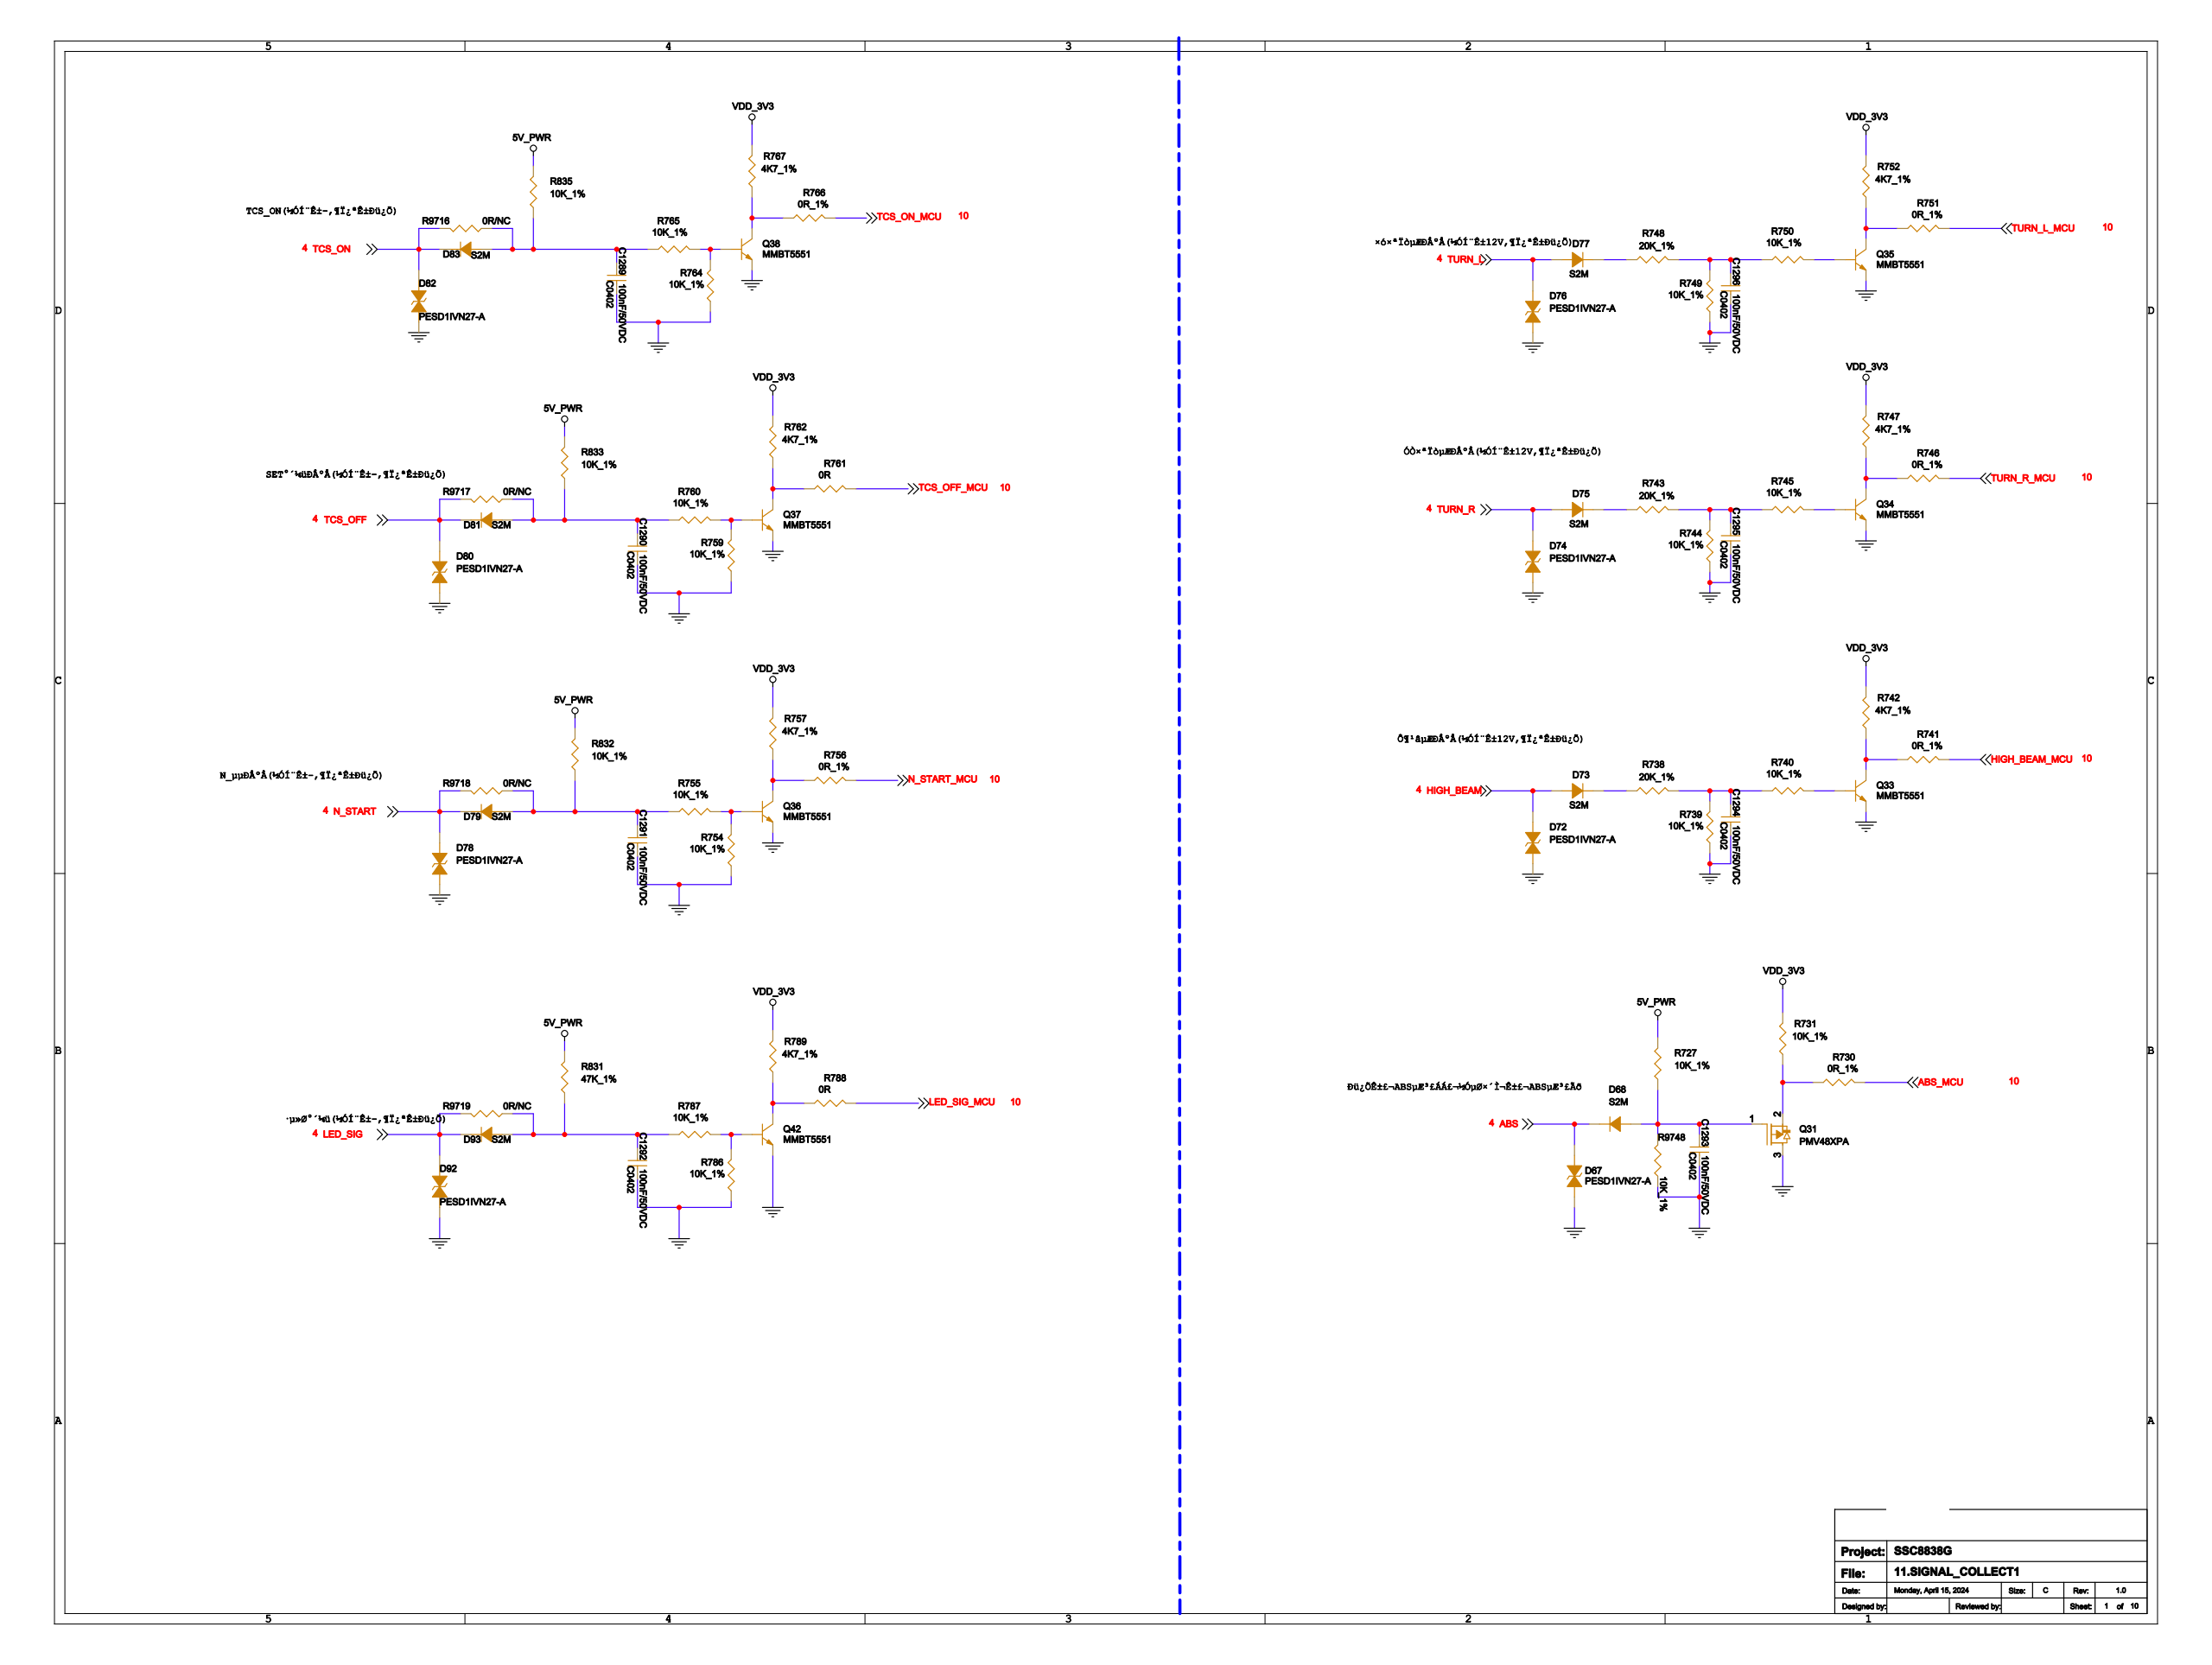Circuit board | Cadence Allegro | 958 parts | 601 nets | one sheet of the schematic
Parts on this sheet (reference | value | footprint):
C1289 | 100nF/50VDC | C0402
C1290 | 100nF/50VDC | C0402
C1291 | 100nF/50VDC | C0402
C1292 | 100nF/50VDC | C0402
C1293 | 100nF/50VDC | C0402
C1294 | 100nF/50VDC | C0402
C1295 | 100nF/50VDC | C0402
C1296 | 100nF/50VDC | C0402
D67 | PESD1IVN27-A | SOD_323
D68 | S2M | DO-214AA
D72 | PESD1IVN27-A | SOD_323
D73 | S2M | DO-214AA
D74 | PESD1IVN27-A | SOD_323
D75 | S2M | DO-214AA
D76 | PESD1IVN27-A | SOD_323
D77 | S2M | DO-214AA
D78 | PESD1IVN27-A | SOD_323
D79 | S2M | DO-214AA
D80 | PESD1IVN27-A | SOD_323
D81 | S2M | DO-214AA
D82 | PESD1IVN27-A | SOD_323
D83 | S2M | DO-214AA
D92 | PESD1IVN27-A | SOD_323
D93 | S2M | DO-214AA
Q31 | PMV48XPA | SOT23-123
Q33 | MMBT5551 | SOT23-123
Q34 | MMBT5551 | SOT23-123
Q35 | MMBT5551 | SOT23-123
Q36 | MMBT5551 | SOT23-123
Q37 | MMBT5551 | SOT23-123
Q38 | MMBT5551 | SOT23-123
Q42 | MMBT5551 | SOT23-123
R727 | 10K_1% | R0402
R730 | 0R_1% | R0402
R731 | 10K_1% | R0402
R738 | 20K_1% | R0402
R739 | 10K_1% | R0402
R740 | 10K_1% | R0402
R741 | 0R_1% | R0402
R742 | 4K7_1% | R0402
R743 | 20K_1% | R0402
R744 | 10K_1% | R0402
R745 | 10K_1% | R0402
R746 | 0R_1% | R0402
R747 | 4K7_1% | R0402
R748 | 20K_1% | R0402
R749 | 10K_1% | R0402
R750 | 10K_1% | R0402
R751 | 0R_1% | R0402
R752 | 4K7_1% | R0402
R754 | 10K_1% | R0402
R755 | 10K_1% | R0402
R756 | 0R_1% | R0402
R757 | 4K7_1% | R0402
R759 | 10K_1% | R0402
R760 | 10K_1% | R0402
R761 | 0R | R0402
R762 | 4K7_1% | R0402
R764 | 10K_1% | R0402
R765 | 10K_1% | R0402
R766 | 0R_1% | R0402
R767 | 4K7_1% | R0402
R786 | 10K_1% | R0402
R787 | 10K_1% | R0402
R788 | 0R | R0402
R789 | 4K7_1% | R0402
R831 | 47K_1% | R0402
R832 | 10K_1% | R0402
R833 | 10K_1% | R0402
R835 | 10K_1% | R0402
R9716 | 0R/NC | R0402
R9717 | 0R/NC | R0402
R9718 | 0R/NC | R0402
R9719 | 0R/NC | R0402
R9748 | 10K_1% | R0402
Nets of these parts (net: part-pin ...):
GND: C1289-2 C1290-2 C1291-2 C1292-2 C1293-2 C1294-2 C1295-2 C1296-2 D67-1 D72-1 D74-1 D76-1 D78-1 D80-1 D82-1 D92-1 Q31-3 Q33-2 Q34-2 Q35-2 Q36-2 Q37-2 Q38-2 Q42-2 R739-1 R744-1 R749-1 R754-1 R759-1 R764-1 R786-1 R9748-1
5V_PWR: R727-2 R831-2 R832-2 R833-2 R835-2
3V3_NORMAL: R731-2 R742-2 R747-2 R752-2 R757-2 R762-2 R767-2 R789-2
N21196393: C1289-1 D83-1 R765-1 R835-1 R9716-1
N21196077: C1290-1 D81-1 R760-1 R833-1 R9717-1
N21195769: C1291-1 D79-1 R755-1 R832-1 R9718-1
N21201066: C1292-1 D93-1 R787-1 R831-1 R9719-1
N21190767: C1293-1 D68-1 Q31-1 R727-1 R9748-2
N21194756: C1294-1 R738-2 R739-2 R740-1
N21195078: C1295-1 R743-2 R744-2 R745-1
N21195469: C1296-1 R748-2 R749-2 R750-1
ABS: D67-2 D68-2
HIGH_BEAM: D72-2 D73-1
TURN_R: D74-2 D75-1
TURN_L: D76-2 D77-1
N_START: D78-2 D79-2 R9718-2
TCS_OFF: D80-2 D81-2 R9717-2
TCS_ON: D82-2 D83-2 R9716-2
LED_SIG: D92-2 D93-2 R9719-2
N21213420: D73-2 R738-1
N21213426: D75-2 R743-1
N21213438: D77-2 R748-1
N21190797: Q31-2 R730-1 R731-1
N21194792: Q33-1 R740-2
N21194816: Q33-3 R741-1 R742-1
N21195114: Q34-1 R745-2
N21195138: Q34-3 R746-1 R747-1
N21195505: Q35-1 R750-2
N21195529: Q35-3 R751-1 R752-1
N21195781: Q36-1 R754-2 R755-2
N21195829: Q36-3 R756-1 R757-1
N21196089: Q37-1 R759-2 R760-2
N21196137: Q37-3 R761-1 R762-1
N21196405: Q38-1 R764-2 R765-2
N21196453: Q38-3 R766-1 R767-1
N21201068: Q42-1 R786-2 R787-2
N21201088: Q42-3 R788-1 R789-1
ABS_MCU: R730-2
HIGH_BEAM_MCU: R741-2
TURN_R_MCU: R746-2
TURN_L_MCU: R751-2
N_START_MCU: R756-2
TCS_ON_MCU: R766-2
TCS_OFF_MCU: R761-2
LED_SIG_MCU: R788-2